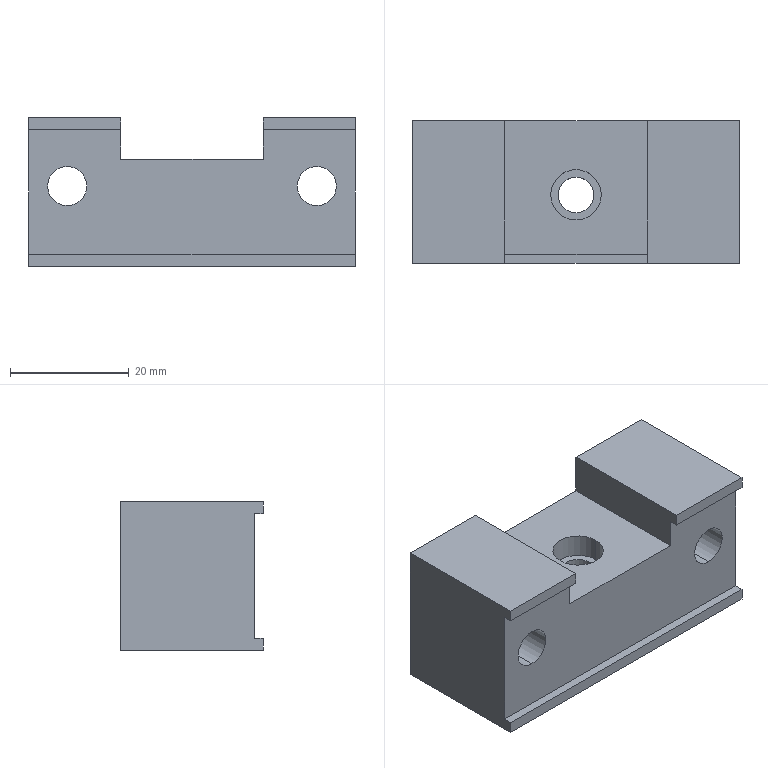Part | STEP file | 11-FG-B02711 | 1 solid | 39 faces | box 55 x 24 x 25 mm | volume 23943 mm3 | plane 21 | cylinder 18 | commonest cylinder face diameters 8.5 x6 6.6 x4 11 x4 4.2 x2 6 x2
STEP:
#1=CARTESIAN_POINT('',(18.75,15.,3.5));
#2=VERTEX_POINT('',#1);
#3=CARTESIAN_POINT('',(10.25,15.,3.5));
#4=VERTEX_POINT('',#3);
#5=CARTESIAN_POINT('',(14.5,15.,3.5));
#6=DIRECTION('',(0.,0.,-1.));
#7=DIRECTION('',(-1.,0.,0.));
#8=AXIS2_PLACEMENT_3D('',#5,#6,#7);
#9=CIRCLE('',#8,4.25);
#10=EDGE_CURVE('',#2,#4,#9,.T.);
#11=ORIENTED_EDGE('',*,*,#10,.F.);
#12=CARTESIAN_POINT('',(18.75,15.,0.));
#13=VERTEX_POINT('',#12);
#14=CARTESIAN_POINT('',(18.75,15.,3.5));
#15=DIRECTION('',(0.,0.,-1.));
#16=VECTOR('',#15,1000.);
#17=LINE('',#14,#16);
#18=EDGE_CURVE('',#2,#13,#17,.T.);
#19=ORIENTED_EDGE('',*,*,#18,.T.);
#20=CARTESIAN_POINT('',(10.25,15.,0.));
#21=VERTEX_POINT('',#20);
#22=CARTESIAN_POINT('',(14.5,15.,0.));
#23=DIRECTION('',(0.,0.,-1.));
#24=DIRECTION('',(-1.,0.,0.));
#25=AXIS2_PLACEMENT_3D('',#22,#23,#24);
#26=CIRCLE('',#25,4.25);
#27=EDGE_CURVE('',#13,#21,#26,.T.);
#28=ORIENTED_EDGE('',*,*,#27,.T.);
#29=CARTESIAN_POINT('',(10.25,15.,3.5));
#30=DIRECTION('',(0.,0.,-1.));
#31=VECTOR('',#30,1000.);
#32=LINE('',#29,#31);
#33=EDGE_CURVE('',#4,#21,#32,.T.);
#34=ORIENTED_EDGE('',*,*,#33,.F.);
#35=EDGE_LOOP('',(#11,#19,#28,#34));
#36=FACE_OUTER_BOUND('',#35,.T.);
#37=CARTESIAN_POINT('',(14.5,15.,3.5));
#38=DIRECTION('',(0.,0.,-1.));
#39=DIRECTION('',(-1.,0.,0.));
#40=AXIS2_PLACEMENT_3D('',#37,#38,#39);
#41=CYLINDRICAL_SURFACE('',#40,4.25);
#42=ADVANCED_FACE('',(#36),#41,.F.);
#43=CARTESIAN_POINT('',(44.75,15.,3.5));
#44=VERTEX_POINT('',#43);
#45=CARTESIAN_POINT('',(36.25,15.,3.5));
#46=VERTEX_POINT('',#45);
#47=CARTESIAN_POINT('',(40.5,15.,3.5));
#48=DIRECTION('',(0.,0.,-1.));
#49=DIRECTION('',(-1.,0.,0.));
#50=AXIS2_PLACEMENT_3D('',#47,#48,#49);
#51=CIRCLE('',#50,4.25);
#52=EDGE_CURVE('',#44,#46,#51,.T.);
#53=ORIENTED_EDGE('',*,*,#52,.F.);
#54=CARTESIAN_POINT('',(44.75,15.,0.));
#55=VERTEX_POINT('',#54);
#56=CARTESIAN_POINT('',(44.75,15.,3.5));
#57=DIRECTION('',(0.,0.,-1.));
#58=VECTOR('',#57,1000.);
#59=LINE('',#56,#58);
#60=EDGE_CURVE('',#44,#55,#59,.T.);
#61=ORIENTED_EDGE('',*,*,#60,.T.);
#62=CARTESIAN_POINT('',(36.25,15.,0.));
#63=VERTEX_POINT('',#62);
#64=CARTESIAN_POINT('',(40.5,15.,0.));
#65=DIRECTION('',(0.,0.,-1.));
#66=DIRECTION('',(-1.,0.,0.));
#67=AXIS2_PLACEMENT_3D('',#64,#65,#66);
#68=CIRCLE('',#67,4.25);
#69=EDGE_CURVE('',#55,#63,#68,.T.);
#70=ORIENTED_EDGE('',*,*,#69,.T.);
#71=CARTESIAN_POINT('',(36.25,15.,3.5));
#72=DIRECTION('',(0.,0.,-1.));
#73=VECTOR('',#72,1000.);
#74=LINE('',#71,#73);
#75=EDGE_CURVE('',#46,#63,#74,.T.);
#76=ORIENTED_EDGE('',*,*,#75,.F.);
#77=EDGE_LOOP('',(#53,#61,#70,#76));
#78=FACE_OUTER_BOUND('',#77,.T.);
#79=CARTESIAN_POINT('',(40.5,15.,3.5));
#80=DIRECTION('',(0.,0.,-1.));
#81=DIRECTION('',(-1.,0.,0.));
#82=AXIS2_PLACEMENT_3D('',#79,#80,#81);
#83=CYLINDRICAL_SURFACE('',#82,4.25);
#84=ADVANCED_FACE('',(#78),#83,.F.);
#85=CARTESIAN_POINT('',(6.5,17.6,8.));
#86=VERTEX_POINT('',#85);
#87=CARTESIAN_POINT('',(6.5,17.6,19.));
#88=VERTEX_POINT('',#87);
#89=CARTESIAN_POINT('',(6.5,17.6,13.5));
#90=DIRECTION('',(0.,1.,0.));
#91=DIRECTION('',(0.,0.,1.));
#92=AXIS2_PLACEMENT_3D('',#89,#90,#91);
#93=CIRCLE('',#92,5.5);
#94=EDGE_CURVE('',#86,#88,#93,.T.);
#95=ORIENTED_EDGE('',*,*,#94,.F.);
#96=CARTESIAN_POINT('',(6.5,24.,8.));
#97=VERTEX_POINT('',#96);
#98=CARTESIAN_POINT('',(6.5,24.,8.));
#99=DIRECTION('',(0.,1.,0.));
#100=VECTOR('',#99,1000.);
#101=LINE('',#98,#100);
#102=EDGE_CURVE('',#86,#97,#101,.T.);
#103=ORIENTED_EDGE('',*,*,#102,.T.);
#104=CARTESIAN_POINT('',(6.5,24.,19.));
#105=VERTEX_POINT('',#104);
#106=CARTESIAN_POINT('',(6.5,24.,13.5));
#107=DIRECTION('',(0.,1.,0.));
#108=DIRECTION('',(0.,0.,1.));
#109=AXIS2_PLACEMENT_3D('',#106,#107,#108);
#110=CIRCLE('',#109,5.5);
#111=EDGE_CURVE('',#97,#105,#110,.T.);
#112=ORIENTED_EDGE('',*,*,#111,.T.);
#113=CARTESIAN_POINT('',(6.5,24.,19.));
#114=DIRECTION('',(0.,1.,0.));
#115=VECTOR('',#114,1000.);
#116=LINE('',#113,#115);
#117=EDGE_CURVE('',#88,#105,#116,.T.);
#118=ORIENTED_EDGE('',*,*,#117,.F.);
#119=EDGE_LOOP('',(#95,#103,#112,#118));
#120=FACE_OUTER_BOUND('',#119,.T.);
#121=CARTESIAN_POINT('',(6.5,24.,13.5));
#122=DIRECTION('',(0.,1.,0.));
#123=DIRECTION('',(0.,0.,1.));
#124=AXIS2_PLACEMENT_3D('',#121,#122,#123);
#125=CYLINDRICAL_SURFACE('',#124,5.5);
#126=ADVANCED_FACE('',(#120),#125,.F.);
#127=CARTESIAN_POINT('',(6.5,1.5,10.2));
#128=VERTEX_POINT('',#127);
#129=CARTESIAN_POINT('',(6.5,1.5,16.8));
#130=VERTEX_POINT('',#129);
#131=CARTESIAN_POINT('',(6.5,1.5,13.5));
#132=DIRECTION('',(0.,1.,0.));
#133=DIRECTION('',(-1.,0.,0.));
#134=AXIS2_PLACEMENT_3D('',#131,#132,#133);
#135=CIRCLE('',#134,3.3);
#136=EDGE_CURVE('',#128,#130,#135,.T.);
#137=ORIENTED_EDGE('',*,*,#136,.F.);
#138=CARTESIAN_POINT('',(6.5,17.6,10.2));
#139=VERTEX_POINT('',#138);
#140=CARTESIAN_POINT('',(6.5,24.,10.2));
#141=DIRECTION('',(0.,1.,0.));
#142=VECTOR('',#141,1000.);
#143=LINE('',#140,#142);
#144=EDGE_CURVE('',#128,#139,#143,.T.);
#145=ORIENTED_EDGE('',*,*,#144,.T.);
#146=CARTESIAN_POINT('',(6.5,17.6,16.8));
#147=VERTEX_POINT('',#146);
#148=CARTESIAN_POINT('',(6.5,17.6,13.5));
#149=DIRECTION('',(0.,1.,0.));
#150=DIRECTION('',(0.,0.,1.));
#151=AXIS2_PLACEMENT_3D('',#148,#149,#150);
#152=CIRCLE('',#151,3.3);
#153=EDGE_CURVE('',#139,#147,#152,.T.);
#154=ORIENTED_EDGE('',*,*,#153,.T.);
#155=CARTESIAN_POINT('',(6.5,24.,16.8));
#156=DIRECTION('',(0.,1.,0.));
#157=VECTOR('',#156,1000.);
#158=LINE('',#155,#157);
#159=EDGE_CURVE('',#130,#147,#158,.T.);
#160=ORIENTED_EDGE('',*,*,#159,.F.);
#161=EDGE_LOOP('',(#137,#145,#154,#160));
#162=FACE_OUTER_BOUND('',#161,.T.);
#163=CARTESIAN_POINT('',(6.5,24.,13.5));
#164=DIRECTION('',(0.,1.,0.));
#165=DIRECTION('',(0.,0.,1.));
#166=AXIS2_PLACEMENT_3D('',#163,#164,#165);
#167=CYLINDRICAL_SURFACE('',#166,3.3);
#168=ADVANCED_FACE('',(#162),#167,.F.);
#169=CARTESIAN_POINT('',(48.5,17.6,8.));
#170=VERTEX_POINT('',#169);
#171=CARTESIAN_POINT('',(48.5,17.6,19.));
#172=VERTEX_POINT('',#171);
#173=CARTESIAN_POINT('',(48.5,17.6,13.5));
#174=DIRECTION('',(0.,1.,0.));
#175=DIRECTION('',(0.,0.,1.));
#176=AXIS2_PLACEMENT_3D('',#173,#174,#175);
#177=CIRCLE('',#176,5.5);
#178=EDGE_CURVE('',#170,#172,#177,.T.);
#179=ORIENTED_EDGE('',*,*,#178,.F.);
#180=CARTESIAN_POINT('',(48.5,24.,8.));
#181=VERTEX_POINT('',#180);
#182=CARTESIAN_POINT('',(48.5,24.,8.));
#183=DIRECTION('',(0.,1.,0.));
#184=VECTOR('',#183,1000.);
#185=LINE('',#182,#184);
#186=EDGE_CURVE('',#170,#181,#185,.T.);
#187=ORIENTED_EDGE('',*,*,#186,.T.);
#188=CARTESIAN_POINT('',(48.5,24.,19.));
#189=VERTEX_POINT('',#188);
#190=CARTESIAN_POINT('',(48.5,24.,13.5));
#191=DIRECTION('',(0.,1.,0.));
#192=DIRECTION('',(0.,0.,1.));
#193=AXIS2_PLACEMENT_3D('',#190,#191,#192);
#194=CIRCLE('',#193,5.5);
#195=EDGE_CURVE('',#181,#189,#194,.T.);
#196=ORIENTED_EDGE('',*,*,#195,.T.);
#197=CARTESIAN_POINT('',(48.5,24.,19.));
#198=DIRECTION('',(0.,1.,0.));
#199=VECTOR('',#198,1000.);
#200=LINE('',#197,#199);
#201=EDGE_CURVE('',#172,#189,#200,.T.);
#202=ORIENTED_EDGE('',*,*,#201,.F.);
#203=EDGE_LOOP('',(#179,#187,#196,#202));
#204=FACE_OUTER_BOUND('',#203,.T.);
#205=CARTESIAN_POINT('',(48.5,24.,13.5));
#206=DIRECTION('',(0.,1.,0.));
#207=DIRECTION('',(0.,0.,1.));
#208=AXIS2_PLACEMENT_3D('',#205,#206,#207);
#209=CYLINDRICAL_SURFACE('',#208,5.5);
#210=ADVANCED_FACE('',(#204),#209,.F.);
#211=CARTESIAN_POINT('',(48.5,1.5,10.2));
#212=VERTEX_POINT('',#211);
#213=CARTESIAN_POINT('',(48.5,1.5,16.8));
#214=VERTEX_POINT('',#213);
#215=CARTESIAN_POINT('',(48.5,1.5,13.5));
#216=DIRECTION('',(0.,1.,0.));
#217=DIRECTION('',(-1.,0.,0.));
#218=AXIS2_PLACEMENT_3D('',#215,#216,#217);
#219=CIRCLE('',#218,3.3);
#220=EDGE_CURVE('',#212,#214,#219,.T.);
#221=ORIENTED_EDGE('',*,*,#220,.F.);
#222=CARTESIAN_POINT('',(48.5,17.6,10.2));
#223=VERTEX_POINT('',#222);
#224=CARTESIAN_POINT('',(48.5,24.,10.2));
#225=DIRECTION('',(0.,1.,0.));
#226=VECTOR('',#225,1000.);
#227=LINE('',#224,#226);
#228=EDGE_CURVE('',#212,#223,#227,.T.);
#229=ORIENTED_EDGE('',*,*,#228,.T.);
#230=CARTESIAN_POINT('',(48.5,17.6,16.8));
#231=VERTEX_POINT('',#230);
#232=CARTESIAN_POINT('',(48.5,17.6,13.5));
#233=DIRECTION('',(0.,1.,0.));
#234=DIRECTION('',(0.,0.,1.));
#235=AXIS2_PLACEMENT_3D('',#232,#233,#234);
#236=CIRCLE('',#235,3.3);
#237=EDGE_CURVE('',#223,#231,#236,.T.);
#238=ORIENTED_EDGE('',*,*,#237,.T.);
#239=CARTESIAN_POINT('',(48.5,24.,16.8));
#240=DIRECTION('',(0.,1.,0.));
#241=VECTOR('',#240,1000.);
#242=LINE('',#239,#241);
#243=EDGE_CURVE('',#214,#231,#242,.T.);
#244=ORIENTED_EDGE('',*,*,#243,.F.);
#245=EDGE_LOOP('',(#221,#229,#238,#244));
#246=FACE_OUTER_BOUND('',#245,.T.);
#247=CARTESIAN_POINT('',(48.5,24.,13.5));
#248=DIRECTION('',(0.,1.,0.));
#249=DIRECTION('',(0.,0.,1.));
#250=AXIS2_PLACEMENT_3D('',#247,#248,#249);
#251=CYLINDRICAL_SURFACE('',#250,3.3);
#252=ADVANCED_FACE('',(#246),#251,.F.);
#253=CARTESIAN_POINT('',(27.5,14.5,2.4));
#254=VERTEX_POINT('',#253);
#255=CARTESIAN_POINT('',(27.5,14.5,6.6));
#256=VERTEX_POINT('',#255);
#257=CARTESIAN_POINT('',(27.5,14.5,2.4));
#258=CARTESIAN_POINT('',(27.358,14.5,2.4));
#259=CARTESIAN_POINT('',(27.214,14.49,2.415));
#260=CARTESIAN_POINT('',(26.936,14.45,2.472));
#261=CARTESIAN_POINT('',(26.803,14.421,2.514));
#262=CARTESIAN_POINT('',(26.419,14.311,2.678));
#263=CARTESIAN_POINT('',(26.194,14.209,2.834));
#264=CARTESIAN_POINT('',(25.915,14.049,3.116));
#265=CARTESIAN_POINT('',(25.831,13.995,3.218));
#266=CARTESIAN_POINT('',(25.683,13.889,3.439));
#267=CARTESIAN_POINT('',(25.618,13.837,3.558));
#268=CARTESIAN_POINT('',(25.513,13.749,3.807));
#269=CARTESIAN_POINT('',(25.471,13.71,3.941));
#270=CARTESIAN_POINT('',(25.414,13.657,4.217));
#271=CARTESIAN_POINT('',(25.4,13.642,4.358));
#272=CARTESIAN_POINT('',(25.4,13.643,4.647));
#273=CARTESIAN_POINT('',(25.415,13.658,4.788));
#274=CARTESIAN_POINT('',(25.472,13.711,5.064));
#275=CARTESIAN_POINT('',(25.515,13.75,5.197));
#276=CARTESIAN_POINT('',(25.673,13.884,5.571));
#277=CARTESIAN_POINT('',(25.824,13.998,5.793));
#278=CARTESIAN_POINT('',(26.105,14.158,6.075));
#279=CARTESIAN_POINT('',(26.209,14.211,6.162));
#280=CARTESIAN_POINT('',(26.431,14.305,6.312));
#281=CARTESIAN_POINT('',(26.549,14.348,6.377));
#282=CARTESIAN_POINT('',(26.803,14.421,6.486));
#283=CARTESIAN_POINT('',(26.939,14.45,6.528));
#284=CARTESIAN_POINT('',(27.214,14.49,6.585));
#285=CARTESIAN_POINT('',(27.356,14.5,6.6));
#286=CARTESIAN_POINT('',(27.5,14.5,6.6));
#287=B_SPLINE_CURVE_WITH_KNOTS('',3,(#257,#258,#259,#260,#261,#262,#263,#264,#265,#266,#267,#268,#269,#270,#271,#272,#273,#274,#275,#276,#277,#278,#279,#280,#281,#282,#283,#284,#285,#286),.UNSPECIFIED.,.F.,.F.,(4,2,2,2,2,2,2,2,2,2,2,2,2,2,4),(0.006821,0.007247,0.007673,0.008524,0.00895,0.009376,0.009801,0.01023,0.01065,0.01108,0.01193,0.01236,0.01278,0.01321,0.01363),.UNSPECIFIED.);
#288=EDGE_CURVE('',#254,#256,#287,.T.);
#289=ORIENTED_EDGE('',*,*,#288,.F.);
#290=CARTESIAN_POINT('',(27.5,24.,2.4));
#291=VERTEX_POINT('',#290);
#292=CARTESIAN_POINT('',(27.5,24.,2.4));
#293=DIRECTION('',(0.,1.,0.));
#294=VECTOR('',#293,1000.);
#295=LINE('',#292,#294);
#296=EDGE_CURVE('',#254,#291,#295,.T.);
#297=ORIENTED_EDGE('',*,*,#296,.T.);
#298=CARTESIAN_POINT('',(27.5,24.,6.6));
#299=VERTEX_POINT('',#298);
#300=CARTESIAN_POINT('',(27.5,24.,4.5));
#301=DIRECTION('',(0.,1.,0.));
#302=DIRECTION('',(0.,0.,1.));
#303=AXIS2_PLACEMENT_3D('',#300,#301,#302);
#304=CIRCLE('',#303,2.1);
#305=EDGE_CURVE('',#291,#299,#304,.T.);
#306=ORIENTED_EDGE('',*,*,#305,.T.);
#307=CARTESIAN_POINT('',(27.5,24.,6.6));
#308=DIRECTION('',(0.,1.,0.));
#309=VECTOR('',#308,1000.);
#310=LINE('',#307,#309);
#311=EDGE_CURVE('',#256,#299,#310,.T.);
#312=ORIENTED_EDGE('',*,*,#311,.F.);
#313=EDGE_LOOP('',(#289,#297,#306,#312));
#314=FACE_OUTER_BOUND('',#313,.T.);
#315=CARTESIAN_POINT('',(27.5,24.,4.5));
#316=DIRECTION('',(0.,1.,0.));
#317=DIRECTION('',(0.,0.,1.));
#318=AXIS2_PLACEMENT_3D('',#315,#316,#317);
#319=CYLINDRICAL_SURFACE('',#318,2.1);
#320=ADVANCED_FACE('',(#314),#319,.F.);
#321=CARTESIAN_POINT('',(23.25,11.5,14.));
#322=VERTEX_POINT('',#321);
#323=CARTESIAN_POINT('',(31.75,11.5,14.));
#324=VERTEX_POINT('',#323);
#325=CARTESIAN_POINT('',(27.5,11.5,14.));
#326=DIRECTION('',(0.,0.,1.));
#327=DIRECTION('',(1.,0.,0.));
#328=AXIS2_PLACEMENT_3D('',#325,#326,#327);
#329=CIRCLE('',#328,4.25);
#330=EDGE_CURVE('',#322,#324,#329,.T.);
#331=ORIENTED_EDGE('',*,*,#330,.F.);
#332=CARTESIAN_POINT('',(23.25,11.5,18.));
#333=VERTEX_POINT('',#332);
#334=CARTESIAN_POINT('',(23.25,11.5,14.));
#335=DIRECTION('',(0.,0.,1.));
#336=VECTOR('',#335,1000.);
#337=LINE('',#334,#336);
#338=EDGE_CURVE('',#322,#333,#337,.T.);
#339=ORIENTED_EDGE('',*,*,#338,.T.);
#340=CARTESIAN_POINT('',(31.75,11.5,18.));
#341=VERTEX_POINT('',#340);
#342=CARTESIAN_POINT('',(27.5,11.5,18.));
#343=DIRECTION('',(0.,0.,1.));
#344=DIRECTION('',(1.,0.,0.));
#345=AXIS2_PLACEMENT_3D('',#342,#343,#344);
#346=CIRCLE('',#345,4.25);
#347=EDGE_CURVE('',#333,#341,#346,.T.);
#348=ORIENTED_EDGE('',*,*,#347,.T.);
#349=CARTESIAN_POINT('',(31.75,11.5,14.));
#350=DIRECTION('',(0.,0.,1.));
#351=VECTOR('',#350,1000.);
#352=LINE('',#349,#351);
#353=EDGE_CURVE('',#324,#341,#352,.T.);
#354=ORIENTED_EDGE('',*,*,#353,.F.);
#355=EDGE_LOOP('',(#331,#339,#348,#354));
#356=FACE_OUTER_BOUND('',#355,.T.);
#357=CARTESIAN_POINT('',(27.5,11.5,14.));
#358=DIRECTION('',(0.,0.,1.));
#359=DIRECTION('',(1.,0.,0.));
#360=AXIS2_PLACEMENT_3D('',#357,#358,#359);
#361=CYLINDRICAL_SURFACE('',#360,4.25);
#362=ADVANCED_FACE('',(#356),#361,.F.);
#363=CARTESIAN_POINT('',(30.5,11.5,0.));
#364=VERTEX_POINT('',#363);
#365=CARTESIAN_POINT('',(24.5,11.5,0.));
#366=VERTEX_POINT('',#365);
#367=CARTESIAN_POINT('',(27.5,11.5,0.));
#368=DIRECTION('',(0.,0.,-1.));
#369=DIRECTION('',(-1.,0.,0.));
#370=AXIS2_PLACEMENT_3D('',#367,#368,#369);
#371=CIRCLE('',#370,3.);
#372=EDGE_CURVE('',#364,#366,#371,.T.);
#373=ORIENTED_EDGE('',*,*,#372,.T.);
#374=CARTESIAN_POINT('',(24.5,11.5,14.));
#375=VERTEX_POINT('',#374);
#376=CARTESIAN_POINT('',(24.5,11.5,-89.));
#377=DIRECTION('',(0.,0.,1.));
#378=VECTOR('',#377,1000.);
#379=LINE('',#376,#378);
#380=EDGE_CURVE('',#366,#375,#379,.T.);
#381=ORIENTED_EDGE('',*,*,#380,.T.);
#382=CARTESIAN_POINT('',(30.5,11.5,14.));
#383=VERTEX_POINT('',#382);
#384=CARTESIAN_POINT('',(27.5,11.5,14.));
#385=DIRECTION('',(0.,0.,-1.));
#386=DIRECTION('',(1.,0.,0.));
#387=AXIS2_PLACEMENT_3D('',#384,#385,#386);
#388=CIRCLE('',#387,3.);
#389=EDGE_CURVE('',#383,#375,#388,.T.);
#390=ORIENTED_EDGE('',*,*,#389,.F.);
#391=CARTESIAN_POINT('',(30.5,11.5,-89.));
#392=DIRECTION('',(0.,0.,1.));
#393=VECTOR('',#392,1000.);
#394=LINE('',#391,#393);
#395=EDGE_CURVE('',#364,#383,#394,.T.);
#396=ORIENTED_EDGE('',*,*,#395,.F.);
#397=EDGE_LOOP('',(#373,#381,#390,#396));
#398=FACE_OUTER_BOUND('',#397,.T.);
#399=CARTESIAN_POINT('',(27.5,11.5,-89.));
#400=DIRECTION('',(0.,0.,1.));
#401=DIRECTION('',(1.,0.,0.));
#402=AXIS2_PLACEMENT_3D('',#399,#400,#401);
#403=CYLINDRICAL_SURFACE('',#402,3.);
#404=ADVANCED_FACE('',(#398),#403,.F.);
#405=ORIENTED_EDGE('',*,*,#380,.F.);
#406=CARTESIAN_POINT('',(27.5,11.5,0.));
#407=DIRECTION('',(0.,0.,-1.));
#408=DIRECTION('',(-1.,0.,0.));
#409=AXIS2_PLACEMENT_3D('',#406,#407,#408);
#410=CIRCLE('',#409,3.);
#411=EDGE_CURVE('',#366,#364,#410,.T.);
#412=ORIENTED_EDGE('',*,*,#411,.T.);
#413=ORIENTED_EDGE('',*,*,#395,.T.);
#414=CARTESIAN_POINT('',(27.5,11.5,14.));
#415=DIRECTION('',(0.,0.,-1.));
#416=DIRECTION('',(1.,0.,0.));
#417=AXIS2_PLACEMENT_3D('',#414,#415,#416);
#418=CIRCLE('',#417,3.);
#419=EDGE_CURVE('',#375,#383,#418,.T.);
#420=ORIENTED_EDGE('',*,*,#419,.F.);
#421=EDGE_LOOP('',(#405,#412,#413,#420));
#422=FACE_OUTER_BOUND('',#421,.T.);
#423=CARTESIAN_POINT('',(27.5,14.5,6.6));
#424=CARTESIAN_POINT('',(27.644,14.5,6.6));
#425=CARTESIAN_POINT('',(27.786,14.49,6.585));
#426=CARTESIAN_POINT('',(28.062,14.45,6.528));
#427=CARTESIAN_POINT('',(28.198,14.421,6.485));
#428=CARTESIAN_POINT('',(28.578,14.312,6.323));
#429=CARTESIAN_POINT('',(28.804,14.21,6.167));
#430=CARTESIAN_POINT('',(29.084,14.05,5.885));
#431=CARTESIAN_POINT('',(29.169,13.995,5.782));
#432=CARTESIAN_POINT('',(29.316,13.889,5.562));
#433=CARTESIAN_POINT('',(29.38,13.839,5.446));
#434=CARTESIAN_POINT('',(29.486,13.75,5.196));
#435=CARTESIAN_POINT('',(29.528,13.711,5.062));
#436=CARTESIAN_POINT('',(29.585,13.657,4.788));
#437=CARTESIAN_POINT('',(29.6,13.642,4.643));
#438=CARTESIAN_POINT('',(29.6,13.642,4.358));
#439=CARTESIAN_POINT('',(29.586,13.657,4.216));
#440=CARTESIAN_POINT('',(29.528,13.711,3.938));
#441=CARTESIAN_POINT('',(29.487,13.749,3.807));
#442=CARTESIAN_POINT('',(29.327,13.884,3.429));
#443=CARTESIAN_POINT('',(29.179,13.996,3.21));
#444=CARTESIAN_POINT('',(28.897,14.157,2.926));
#445=CARTESIAN_POINT('',(28.795,14.209,2.841));
#446=CARTESIAN_POINT('',(28.573,14.304,2.69));
#447=CARTESIAN_POINT('',(28.453,14.348,2.624));
#448=CARTESIAN_POINT('',(28.198,14.421,2.514));
#449=CARTESIAN_POINT('',(28.064,14.45,2.472));
#450=CARTESIAN_POINT('',(27.787,14.49,2.415));
#451=CARTESIAN_POINT('',(27.642,14.5,2.4));
#452=CARTESIAN_POINT('',(27.5,14.5,2.4));
#453=B_SPLINE_CURVE_WITH_KNOTS('',3,(#423,#424,#425,#426,#427,#428,#429,#430,#431,#432,#433,#434,#435,#436,#437,#438,#439,#440,#441,#442,#443,#444,#445,#446,#447,#448,#449,#450,#451,#452),.UNSPECIFIED.,.F.,.F.,(4,2,2,2,2,2,2,2,2,2,2,2,2,2,4),(0.,0.0004263,0.0008526,0.001705,0.002132,0.002558,0.002984,0.003411,0.003837,0.004263,0.005116,0.005542,0.005969,0.006395,0.006821),.UNSPECIFIED.);
#454=EDGE_CURVE('',#256,#254,#453,.T.);
#455=ORIENTED_EDGE('',*,*,#454,.T.);
#456=ORIENTED_EDGE('',*,*,#288,.T.);
#457=EDGE_LOOP('',(#455,#456));
#458=FACE_BOUND('',#457,.T.);
#459=CARTESIAN_POINT('',(27.5,11.5,-89.));
#460=DIRECTION('',(0.,0.,1.));
#461=DIRECTION('',(1.,0.,0.));
#462=AXIS2_PLACEMENT_3D('',#459,#460,#461);
#463=CYLINDRICAL_SURFACE('',#462,3.);
#464=ADVANCED_FACE('',(#422,#458),#463,.F.);
#465=CARTESIAN_POINT('',(39.5,0.,25.));
#466=VERTEX_POINT('',#465);
#467=CARTESIAN_POINT('',(55.,0.,25.));
#468=VERTEX_POINT('',#467);
#469=CARTESIAN_POINT('',(0.,0.,25.));
#470=DIRECTION('',(1.,0.,0.));
#471=VECTOR('',#470,1000.);
#472=LINE('',#469,#471);
#473=EDGE_CURVE('',#466,#468,#472,.T.);
#474=ORIENTED_EDGE('',*,*,#473,.F.);
#475=CARTESIAN_POINT('',(39.5,0.,23.));
#476=VERTEX_POINT('',#475);
#477=CARTESIAN_POINT('',(39.5,0.,25.));
#478=DIRECTION('',(0.,0.,-1.));
#479=VECTOR('',#478,1000.);
#480=LINE('',#477,#479);
#481=EDGE_CURVE('',#466,#476,#480,.T.);
#482=ORIENTED_EDGE('',*,*,#481,.T.);
#483=CARTESIAN_POINT('',(55.,0.,23.));
#484=VERTEX_POINT('',#483);
#485=CARTESIAN_POINT('',(107.,0.,23.));
#486=DIRECTION('',(-1.,0.,0.));
#487=VECTOR('',#486,1000.);
#488=LINE('',#485,#487);
#489=EDGE_CURVE('',#484,#476,#488,.T.);
#490=ORIENTED_EDGE('',*,*,#489,.F.);
#491=CARTESIAN_POINT('',(55.,0.,25.));
#492=DIRECTION('',(0.,0.,-1.));
#493=VECTOR('',#492,1000.);
#494=LINE('',#491,#493);
#495=EDGE_CURVE('',#468,#484,#494,.T.);
#496=ORIENTED_EDGE('',*,*,#495,.F.);
#497=EDGE_LOOP('',(#474,#482,#490,#496));
#498=FACE_OUTER_BOUND('',#497,.T.);
#499=CARTESIAN_POINT('',(0.,0.,25.));
#500=DIRECTION('',(0.,1.,0.));
#501=DIRECTION('',(0.,0.,1.));
#502=AXIS2_PLACEMENT_3D('',#499,#500,#501);
#503=PLANE('',#502);
#504=ADVANCED_FACE('',(#498),#503,.F.);
#505=CARTESIAN_POINT('',(55.,24.,25.));
#506=VERTEX_POINT('',#505);
#507=CARTESIAN_POINT('',(39.5,24.,25.));
#508=VERTEX_POINT('',#507);
#509=CARTESIAN_POINT('',(0.,24.,25.));
#510=DIRECTION('',(-1.,0.,0.));
#511=VECTOR('',#510,1000.);
#512=LINE('',#509,#511);
#513=EDGE_CURVE('',#506,#508,#512,.T.);
#514=ORIENTED_EDGE('',*,*,#513,.T.);
#515=CARTESIAN_POINT('',(39.5,-83.,25.));
#516=DIRECTION('',(0.,1.,0.));
#517=VECTOR('',#516,1000.);
#518=LINE('',#515,#517);
#519=EDGE_CURVE('',#466,#508,#518,.T.);
#520=ORIENTED_EDGE('',*,*,#519,.F.);
#521=ORIENTED_EDGE('',*,*,#473,.T.);
#522=CARTESIAN_POINT('',(55.,0.,25.));
#523=DIRECTION('',(0.,1.,0.));
#524=VECTOR('',#523,1000.);
#525=LINE('',#522,#524);
#526=EDGE_CURVE('',#468,#506,#525,.T.);
#527=ORIENTED_EDGE('',*,*,#526,.T.);
#528=EDGE_LOOP('',(#514,#520,#521,#527));
#529=FACE_OUTER_BOUND('',#528,.T.);
#530=CARTESIAN_POINT('',(0.,24.,25.));
#531=DIRECTION('',(0.,0.,-1.));
#532=DIRECTION('',(-1.,0.,0.));
#533=AXIS2_PLACEMENT_3D('',#530,#531,#532);
#534=PLANE('',#533);
#535=ADVANCED_FACE('',(#529),#534,.F.);
#536=ORIENTED_EDGE('',*,*,#489,.T.);
#537=CARTESIAN_POINT('',(39.5,1.5,23.));
#538=VERTEX_POINT('',#537);
#539=CARTESIAN_POINT('',(39.5,0.,23.));
#540=DIRECTION('',(0.,1.,0.));
#541=VECTOR('',#540,1000.);
#542=LINE('',#539,#541);
#543=EDGE_CURVE('',#476,#538,#542,.T.);
#544=ORIENTED_EDGE('',*,*,#543,.T.);
#545=CARTESIAN_POINT('',(55.,1.5,23.));
#546=VERTEX_POINT('',#545);
#547=CARTESIAN_POINT('',(107.,1.5,23.));
#548=DIRECTION('',(-1.,0.,0.));
#549=VECTOR('',#548,1000.);
#550=LINE('',#547,#549);
#551=EDGE_CURVE('',#546,#538,#550,.T.);
#552=ORIENTED_EDGE('',*,*,#551,.F.);
#553=CARTESIAN_POINT('',(55.,0.,23.));
#554=DIRECTION('',(0.,1.,0.));
#555=VECTOR('',#554,1000.);
#556=LINE('',#553,#555);
#557=EDGE_CURVE('',#484,#546,#556,.T.);
#558=ORIENTED_EDGE('',*,*,#557,.F.);
#559=EDGE_LOOP('',(#536,#544,#552,#558));
#560=FACE_OUTER_BOUND('',#559,.T.);
#561=CARTESIAN_POINT('',(107.,0.,23.));
#562=DIRECTION('',(0.,0.,1.));
#563=DIRECTION('',(1.,0.,0.));
#564=AXIS2_PLACEMENT_3D('',#561,#562,#563);
#565=PLANE('',#564);
#566=ADVANCED_FACE('',(#560),#565,.F.);
#567=CARTESIAN_POINT('',(15.5,0.,23.));
#568=VERTEX_POINT('',#567);
#569=CARTESIAN_POINT('',(0.,0.,23.));
#570=VERTEX_POINT('',#569);
#571=CARTESIAN_POINT('',(107.,0.,23.));
#572=DIRECTION('',(-1.,0.,0.));
#573=VECTOR('',#572,1000.);
#574=LINE('',#571,#573);
#575=EDGE_CURVE('',#568,#570,#574,.T.);
#576=ORIENTED_EDGE('',*,*,#575,.F.);
#577=CARTESIAN_POINT('',(15.5,0.,25.));
#578=VERTEX_POINT('',#577);
#579=CARTESIAN_POINT('',(15.5,0.,25.));
#580=DIRECTION('',(0.,0.,1.));
#581=VECTOR('',#580,1000.);
#582=LINE('',#579,#581);
#583=EDGE_CURVE('',#568,#578,#582,.T.);
#584=ORIENTED_EDGE('',*,*,#583,.T.);
#585=CARTESIAN_POINT('',(0.,0.,25.));
#586=VERTEX_POINT('',#585);
#587=CARTESIAN_POINT('',(0.,0.,25.));
#588=DIRECTION('',(1.,0.,0.));
#589=VECTOR('',#588,1000.);
#590=LINE('',#587,#589);
#591=EDGE_CURVE('',#586,#578,#590,.T.);
#592=ORIENTED_EDGE('',*,*,#591,.F.);
#593=CARTESIAN_POINT('',(0.,0.,25.));
#594=DIRECTION('',(0.,0.,-1.));
#595=VECTOR('',#594,1000.);
#596=LINE('',#593,#595);
#597=EDGE_CURVE('',#586,#570,#596,.T.);
#598=ORIENTED_EDGE('',*,*,#597,.T.);
#599=EDGE_LOOP('',(#576,#584,#592,#598));
#600=FACE_OUTER_BOUND('',#599,.T.);
#601=CARTESIAN_POINT('',(0.,0.,25.));
#602=DIRECTION('',(0.,1.,0.));
#603=DIRECTION('',(0.,0.,1.));
#604=AXIS2_PLACEMENT_3D('',#601,#602,#603);
#605=PLANE('',#604);
#606=ADVANCED_FACE('',(#600),#605,.F.);
#607=CARTESIAN_POINT('',(0.,1.5,23.));
#608=VERTEX_POINT('',#607);
#609=CARTESIAN_POINT('',(0.,1.5,2.));
#610=VERTEX_POINT('',#609);
#611=CARTESIAN_POINT('',(0.,1.5,23.));
#612=DIRECTION('',(0.,0.,-1.));
#613=VECTOR('',#612,1000.);
#614=LINE('',#611,#613);
#615=EDGE_CURVE('',#608,#610,#614,.T.);
#616=ORIENTED_EDGE('',*,*,#615,.F.);
#617=CARTESIAN_POINT('',(0.,0.,23.));
#618=DIRECTION('',(0.,1.,0.));
#619=VECTOR('',#618,1000.);
#620=LINE('',#617,#619);
#621=EDGE_CURVE('',#570,#608,#620,.T.);
#622=ORIENTED_EDGE('',*,*,#621,.F.);
#623=ORIENTED_EDGE('',*,*,#597,.F.);
#624=CARTESIAN_POINT('',(0.,24.,25.));
#625=VERTEX_POINT('',#624);
#626=CARTESIAN_POINT('',(0.,0.,25.));
#627=DIRECTION('',(0.,-1.,0.));
#628=VECTOR('',#627,1000.);
#629=LINE('',#626,#628);
#630=EDGE_CURVE('',#625,#586,#629,.T.);
#631=ORIENTED_EDGE('',*,*,#630,.F.);
#632=CARTESIAN_POINT('',(0.,24.,0.));
#633=VERTEX_POINT('',#632);
#634=CARTESIAN_POINT('',(0.,24.,25.));
#635=DIRECTION('',(0.,0.,-1.));
#636=VECTOR('',#635,1000.);
#637=LINE('',#634,#636);
#638=EDGE_CURVE('',#625,#633,#637,.T.);
#639=ORIENTED_EDGE('',*,*,#638,.T.);
#640=CARTESIAN_POINT('',(0.,0.,0.));
#641=VERTEX_POINT('',#640);
#642=CARTESIAN_POINT('',(0.,0.,0.));
#643=DIRECTION('',(0.,-1.,0.));
#644=VECTOR('',#643,1000.);
#645=LINE('',#642,#644);
#646=EDGE_CURVE('',#633,#641,#645,.T.);
#647=ORIENTED_EDGE('',*,*,#646,.T.);
#648=CARTESIAN_POINT('',(0.,0.,2.));
#649=VERTEX_POINT('',#648);
#650=CARTESIAN_POINT('',(0.,0.,25.));
#651=DIRECTION('',(0.,0.,-1.));
#652=VECTOR('',#651,1000.);
#653=LINE('',#650,#652);
#654=EDGE_CURVE('',#649,#641,#653,.T.);
#655=ORIENTED_EDGE('',*,*,#654,.F.);
#656=CARTESIAN_POINT('',(0.,0.,2.));
#657=DIRECTION('',(0.,-1.,0.));
#658=VECTOR('',#657,1000.);
#659=LINE('',#656,#658);
#660=EDGE_CURVE('',#610,#649,#659,.T.);
#661=ORIENTED_EDGE('',*,*,#660,.F.);
#662=EDGE_LOOP('',(#616,#622,#623,#631,#639,#647,#655,#661));
#663=FACE_OUTER_BOUND('',#662,.T.);
#664=CARTESIAN_POINT('',(0.,0.,25.));
#665=DIRECTION('',(1.,0.,0.));
#666=DIRECTION('',(0.,1.,0.));
#667=AXIS2_PLACEMENT_3D('',#664,#665,#666);
#668=PLANE('',#667);
#669=ADVANCED_FACE('',(#663),#668,.F.);
#670=CARTESIAN_POINT('',(55.,0.,2.));
#671=VERTEX_POINT('',#670);
#672=CARTESIAN_POINT('',(55.,0.,0.));
#673=VERTEX_POINT('',#672);
#674=CARTESIAN_POINT('',(55.,0.,25.));
#675=DIRECTION('',(0.,0.,-1.));
#676=VECTOR('',#675,1000.);
#677=LINE('',#674,#676);
#678=EDGE_CURVE('',#671,#673,#677,.T.);
#679=ORIENTED_EDGE('',*,*,#678,.F.);
#680=CARTESIAN_POINT('',(107.,0.,2.));
#681=DIRECTION('',(-1.,0.,0.));
#682=VECTOR('',#681,1000.);
#683=LINE('',#680,#682);
#684=EDGE_CURVE('',#671,#649,#683,.T.);
#685=ORIENTED_EDGE('',*,*,#684,.T.);
#686=ORIENTED_EDGE('',*,*,#654,.T.);
#687=CARTESIAN_POINT('',(0.,0.,0.));
#688=DIRECTION('',(1.,0.,0.));
#689=VECTOR('',#688,1000.);
#690=LINE('',#687,#689);
#691=EDGE_CURVE('',#641,#673,#690,.T.);
#692=ORIENTED_EDGE('',*,*,#691,.T.);
#693=EDGE_LOOP('',(#679,#685,#686,#692));
#694=FACE_OUTER_BOUND('',#693,.T.);
#695=CARTESIAN_POINT('',(0.,0.,25.));
#696=DIRECTION('',(0.,1.,0.));
#697=DIRECTION('',(0.,0.,1.));
#698=AXIS2_PLACEMENT_3D('',#695,#696,#697);
#699=PLANE('',#698);
#700=ADVANCED_FACE('',(#694),#699,.F.);
#701=ORIENTED_EDGE('',*,*,#495,.T.);
#702=ORIENTED_EDGE('',*,*,#557,.T.);
#703=CARTESIAN_POINT('',(55.,1.5,2.));
#704=VERTEX_POINT('',#703);
#705=CARTESIAN_POINT('',(55.,1.5,25.));
#706=DIRECTION('',(0.,0.,-1.));
#707=VECTOR('',#706,1000.);
#708=LINE('',#705,#707);
#709=EDGE_CURVE('',#546,#704,#708,.T.);
#710=ORIENTED_EDGE('',*,*,#709,.T.);
#711=CARTESIAN_POINT('',(55.,0.,2.));
#712=DIRECTION('',(0.,-1.,0.));
#713=VECTOR('',#712,1000.);
#714=LINE('',#711,#713);
#715=EDGE_CURVE('',#704,#671,#714,.T.);
#716=ORIENTED_EDGE('',*,*,#715,.T.);
#717=ORIENTED_EDGE('',*,*,#678,.T.);
#718=CARTESIAN_POINT('',(55.,24.,0.));
#719=VERTEX_POINT('',#718);
#720=CARTESIAN_POINT('',(55.,0.,0.));
#721=DIRECTION('',(0.,1.,0.));
#722=VECTOR('',#721,1000.);
#723=LINE('',#720,#722);
#724=EDGE_CURVE('',#673,#719,#723,.T.);
#725=ORIENTED_EDGE('',*,*,#724,.T.);
#726=CARTESIAN_POINT('',(55.,24.,25.));
#727=DIRECTION('',(0.,0.,-1.));
#728=VECTOR('',#727,1000.);
#729=LINE('',#726,#728);
#730=EDGE_CURVE('',#506,#719,#729,.T.);
#731=ORIENTED_EDGE('',*,*,#730,.F.);
#732=ORIENTED_EDGE('',*,*,#526,.F.);
#733=EDGE_LOOP('',(#701,#702,#710,#716,#717,#725,#731,#732));
#734=FACE_OUTER_BOUND('',#733,.T.);
#735=CARTESIAN_POINT('',(55.,0.,25.));
#736=DIRECTION('',(-1.,0.,0.));
#737=DIRECTION('',(0.,-1.,0.));
#738=AXIS2_PLACEMENT_3D('',#735,#736,#737);
#739=PLANE('',#738);
#740=ADVANCED_FACE('',(#734),#739,.F.);
#741=CARTESIAN_POINT('',(6.5,24.,13.5));
#742=DIRECTION('',(0.,1.,0.));
#743=DIRECTION('',(0.,0.,1.));
#744=AXIS2_PLACEMENT_3D('',#741,#742,#743);
#745=CIRCLE('',#744,5.5);
#746=EDGE_CURVE('',#105,#97,#745,.T.);
#747=ORIENTED_EDGE('',*,*,#746,.F.);
#748=ORIENTED_EDGE('',*,*,#111,.F.);
#749=EDGE_LOOP('',(#747,#748));
#750=FACE_BOUND('',#749,.T.);
#751=CARTESIAN_POINT('',(48.5,24.,13.5));
#752=DIRECTION('',(0.,1.,0.));
#753=DIRECTION('',(0.,0.,1.));
#754=AXIS2_PLACEMENT_3D('',#751,#752,#753);
#755=CIRCLE('',#754,5.5);
#756=EDGE_CURVE('',#189,#181,#755,.T.);
#757=ORIENTED_EDGE('',*,*,#756,.F.);
#758=ORIENTED_EDGE('',*,*,#195,.F.);
#759=EDGE_LOOP('',(#757,#758));
#760=FACE_BOUND('',#759,.T.);
#761=CARTESIAN_POINT('',(27.5,24.,4.5));
#762=DIRECTION('',(0.,1.,0.));
#763=DIRECTION('',(0.,0.,1.));
#764=AXIS2_PLACEMENT_3D('',#761,#762,#763);
#765=CIRCLE('',#764,2.1);
#766=EDGE_CURVE('',#299,#291,#765,.T.);
#767=ORIENTED_EDGE('',*,*,#766,.F.);
#768=ORIENTED_EDGE('',*,*,#305,.F.);
#769=EDGE_LOOP('',(#767,#768));
#770=FACE_BOUND('',#769,.T.);
#771=CARTESIAN_POINT('',(39.5,24.,18.));
#772=VERTEX_POINT('',#771);
#773=CARTESIAN_POINT('',(15.5,24.,18.));
#774=VERTEX_POINT('',#773);
#775=CARTESIAN_POINT('',(39.5,24.,18.));
#776=DIRECTION('',(-1.,0.,0.));
#777=VECTOR('',#776,1000.);
#778=LINE('',#775,#777);
#779=EDGE_CURVE('',#772,#774,#778,.T.);
#780=ORIENTED_EDGE('',*,*,#779,.F.);
#781=CARTESIAN_POINT('',(39.5,24.,25.));
#782=DIRECTION('',(0.,0.,-1.));
#783=VECTOR('',#782,1000.);
#784=LINE('',#781,#783);
#785=EDGE_CURVE('',#508,#772,#784,.T.);
#786=ORIENTED_EDGE('',*,*,#785,.F.);
#787=ORIENTED_EDGE('',*,*,#513,.F.);
#788=ORIENTED_EDGE('',*,*,#730,.T.);
#789=CARTESIAN_POINT('',(0.,24.,0.));
#790=DIRECTION('',(-1.,0.,0.));
#791=VECTOR('',#790,1000.);
#792=LINE('',#789,#791);
#793=EDGE_CURVE('',#719,#633,#792,.T.);
#794=ORIENTED_EDGE('',*,*,#793,.T.);
#795=ORIENTED_EDGE('',*,*,#638,.F.);
#796=CARTESIAN_POINT('',(15.5,24.,25.));
#797=VERTEX_POINT('',#796);
#798=CARTESIAN_POINT('',(0.,24.,25.));
#799=DIRECTION('',(-1.,0.,0.));
#800=VECTOR('',#799,1000.);
#801=LINE('',#798,#800);
#802=EDGE_CURVE('',#797,#625,#801,.T.);
#803=ORIENTED_EDGE('',*,*,#802,.F.);
#804=CARTESIAN_POINT('',(15.5,24.,25.));
#805=DIRECTION('',(0.,0.,1.));
#806=VECTOR('',#805,1000.);
#807=LINE('',#804,#806);
#808=EDGE_CURVE('',#774,#797,#807,.T.);
#809=ORIENTED_EDGE('',*,*,#808,.F.);
#810=EDGE_LOOP('',(#780,#786,#787,#788,#794,#795,#803,#809));
#811=FACE_OUTER_BOUND('',#810,.T.);
#812=CARTESIAN_POINT('',(0.,24.,25.));
#813=DIRECTION('',(0.,-1.,0.));
#814=DIRECTION('',(0.,0.,-1.));
#815=AXIS2_PLACEMENT_3D('',#812,#813,#814);
#816=PLANE('',#815);
#817=ADVANCED_FACE('',(#750,#760,#770,#811),#816,.F.);
#818=ORIENTED_EDGE('',*,*,#591,.T.);
#819=CARTESIAN_POINT('',(15.5,-83.,25.));
#820=DIRECTION('',(0.,1.,0.));
#821=VECTOR('',#820,1000.);
#822=LINE('',#819,#821);
#823=EDGE_CURVE('',#578,#797,#822,.T.);
#824=ORIENTED_EDGE('',*,*,#823,.T.);
#825=ORIENTED_EDGE('',*,*,#802,.T.);
#826=ORIENTED_EDGE('',*,*,#630,.T.);
#827=EDGE_LOOP('',(#818,#824,#825,#826));
#828=FACE_OUTER_BOUND('',#827,.T.);
#829=CARTESIAN_POINT('',(0.,24.,25.));
#830=DIRECTION('',(0.,0.,-1.));
#831=DIRECTION('',(-1.,0.,0.));
#832=AXIS2_PLACEMENT_3D('',#829,#830,#831);
#833=PLANE('',#832);
#834=ADVANCED_FACE('',(#828),#833,.F.);
#835=CARTESIAN_POINT('',(14.5,15.,0.));
#836=DIRECTION('',(0.,0.,-1.));
#837=DIRECTION('',(-1.,0.,0.));
#838=AXIS2_PLACEMENT_3D('',#835,#836,#837);
#839=CIRCLE('',#838,4.25);
#840=EDGE_CURVE('',#21,#13,#839,.T.);
#841=ORIENTED_EDGE('',*,*,#840,.F.);
#842=ORIENTED_EDGE('',*,*,#27,.F.);
#843=EDGE_LOOP('',(#841,#842));
#844=FACE_BOUND('',#843,.T.);
#845=CARTESIAN_POINT('',(40.5,15.,0.));
#846=DIRECTION('',(0.,0.,-1.));
#847=DIRECTION('',(-1.,0.,0.));
#848=AXIS2_PLACEMENT_3D('',#845,#846,#847);
#849=CIRCLE('',#848,4.25);
#850=EDGE_CURVE('',#63,#55,#849,.T.);
#851=ORIENTED_EDGE('',*,*,#850,.F.);
#852=ORIENTED_EDGE('',*,*,#69,.F.);
#853=EDGE_LOOP('',(#851,#852));
#854=FACE_BOUND('',#853,.T.);
#855=ORIENTED_EDGE('',*,*,#372,.F.);
#856=ORIENTED_EDGE('',*,*,#411,.F.);
#857=EDGE_LOOP('',(#855,#856));
#858=FACE_BOUND('',#857,.T.);
#859=ORIENTED_EDGE('',*,*,#646,.F.);
#860=ORIENTED_EDGE('',*,*,#793,.F.);
#861=ORIENTED_EDGE('',*,*,#724,.F.);
#862=ORIENTED_EDGE('',*,*,#691,.F.);
#863=EDGE_LOOP('',(#859,#860,#861,#862));
#864=FACE_OUTER_BOUND('',#863,.T.);
#865=CARTESIAN_POINT('',(0.,24.,0.));
#866=DIRECTION('',(0.,0.,-1.));
#867=DIRECTION('',(-1.,0.,0.));
#868=AXIS2_PLACEMENT_3D('',#865,#866,#867);
#869=PLANE('',#868);
#870=ADVANCED_FACE('',(#844,#854,#858,#864),#869,.T.);
#871=CARTESIAN_POINT('',(15.5,1.5,23.));
#872=VERTEX_POINT('',#871);
#873=CARTESIAN_POINT('',(107.,1.5,23.));
#874=DIRECTION('',(-1.,0.,0.));
#875=VECTOR('',#874,1000.);
#876=LINE('',#873,#875);
#877=EDGE_CURVE('',#872,#608,#876,.T.);
#878=ORIENTED_EDGE('',*,*,#877,.F.);
#879=CARTESIAN_POINT('',(15.5,0.,23.));
#880=DIRECTION('',(0.,-1.,0.));
#881=VECTOR('',#880,1000.);
#882=LINE('',#879,#881);
#883=EDGE_CURVE('',#872,#568,#882,.T.);
#884=ORIENTED_EDGE('',*,*,#883,.T.);
#885=ORIENTED_EDGE('',*,*,#575,.T.);
#886=ORIENTED_EDGE('',*,*,#621,.T.);
#887=EDGE_LOOP('',(#878,#884,#885,#886));
#888=FACE_OUTER_BOUND('',#887,.T.);
#889=CARTESIAN_POINT('',(107.,0.,23.));
#890=DIRECTION('',(0.,0.,1.));
#891=DIRECTION('',(1.,0.,0.));
#892=AXIS2_PLACEMENT_3D('',#889,#890,#891);
#893=PLANE('',#892);
#894=ADVANCED_FACE('',(#888),#893,.F.);
#895=CARTESIAN_POINT('',(107.,1.5,2.));
#896=DIRECTION('',(-1.,0.,0.));
#897=VECTOR('',#896,1000.);
#898=LINE('',#895,#897);
#899=EDGE_CURVE('',#704,#610,#898,.T.);
#900=ORIENTED_EDGE('',*,*,#899,.T.);
#901=ORIENTED_EDGE('',*,*,#660,.T.);
#902=ORIENTED_EDGE('',*,*,#684,.F.);
#903=ORIENTED_EDGE('',*,*,#715,.F.);
#904=EDGE_LOOP('',(#900,#901,#902,#903));
#905=FACE_OUTER_BOUND('',#904,.T.);
#906=CARTESIAN_POINT('',(107.,0.,2.));
#907=DIRECTION('',(0.,0.,-1.));
#908=DIRECTION('',(-1.,0.,0.));
#909=AXIS2_PLACEMENT_3D('',#906,#907,#908);
#910=PLANE('',#909);
#911=ADVANCED_FACE('',(#905),#910,.F.);
#912=CARTESIAN_POINT('',(6.5,1.5,13.5));
#913=DIRECTION('',(0.,1.,0.));
#914=DIRECTION('',(-1.,0.,0.));
#915=AXIS2_PLACEMENT_3D('',#912,#913,#914);
#916=CIRCLE('',#915,3.3);
#917=EDGE_CURVE('',#130,#128,#916,.T.);
#918=ORIENTED_EDGE('',*,*,#917,.T.);
#919=ORIENTED_EDGE('',*,*,#136,.T.);
#920=EDGE_LOOP('',(#918,#919));
#921=FACE_BOUND('',#920,.T.);
#922=CARTESIAN_POINT('',(48.5,1.5,13.5));
#923=DIRECTION('',(0.,1.,0.));
#924=DIRECTION('',(-1.,0.,0.));
#925=AXIS2_PLACEMENT_3D('',#922,#923,#924);
#926=CIRCLE('',#925,3.3);
#927=EDGE_CURVE('',#214,#212,#926,.T.);
#928=ORIENTED_EDGE('',*,*,#927,.T.);
#929=ORIENTED_EDGE('',*,*,#220,.T.);
#930=EDGE_LOOP('',(#928,#929));
#931=FACE_BOUND('',#930,.T.);
#932=ORIENTED_EDGE('',*,*,#551,.T.);
#933=CARTESIAN_POINT('',(39.5,1.5,18.));
#934=VERTEX_POINT('',#933);
#935=CARTESIAN_POINT('',(39.5,1.5,23.));
#936=DIRECTION('',(0.,0.,-1.));
#937=VECTOR('',#936,1000.);
#938=LINE('',#935,#937);
#939=EDGE_CURVE('',#538,#934,#938,.T.);
#940=ORIENTED_EDGE('',*,*,#939,.T.);
#941=CARTESIAN_POINT('',(15.5,1.5,18.));
#942=VERTEX_POINT('',#941);
#943=CARTESIAN_POINT('',(107.,1.5,18.));
#944=DIRECTION('',(-1.,0.,0.));
#945=VECTOR('',#944,1000.);
#946=LINE('',#943,#945);
#947=EDGE_CURVE('',#934,#942,#946,.T.);
#948=ORIENTED_EDGE('',*,*,#947,.T.);
#949=CARTESIAN_POINT('',(15.5,1.5,23.));
#950=DIRECTION('',(0.,0.,1.));
#951=VECTOR('',#950,1000.);
#952=LINE('',#949,#951);
#953=EDGE_CURVE('',#942,#872,#952,.T.);
#954=ORIENTED_EDGE('',*,*,#953,.T.);
#955=ORIENTED_EDGE('',*,*,#877,.T.);
#956=ORIENTED_EDGE('',*,*,#615,.T.);
#957=ORIENTED_EDGE('',*,*,#899,.F.);
#958=ORIENTED_EDGE('',*,*,#709,.F.);
#959=EDGE_LOOP('',(#932,#940,#948,#954,#955,#956,#957,#958));
#960=FACE_OUTER_BOUND('',#959,.T.);
#961=CARTESIAN_POINT('',(107.,1.5,23.));
#962=DIRECTION('',(0.,1.,0.));
#963=DIRECTION('',(-1.,0.,0.));
#964=AXIS2_PLACEMENT_3D('',#961,#962,#963);
#965=PLANE('',#964);
#966=ADVANCED_FACE('',(#921,#931,#960),#965,.F.);
#967=ORIENTED_EDGE('',*,*,#519,.T.);
#968=ORIENTED_EDGE('',*,*,#785,.T.);
#969=CARTESIAN_POINT('',(39.5,-83.,18.));
#970=DIRECTION('',(0.,1.,0.));
#971=VECTOR('',#970,1000.);
#972=LINE('',#969,#971);
#973=EDGE_CURVE('',#934,#772,#972,.T.);
#974=ORIENTED_EDGE('',*,*,#973,.F.);
#975=ORIENTED_EDGE('',*,*,#939,.F.);
#976=ORIENTED_EDGE('',*,*,#543,.F.);
#977=ORIENTED_EDGE('',*,*,#481,.F.);
#978=EDGE_LOOP('',(#967,#968,#974,#975,#976,#977));
#979=FACE_OUTER_BOUND('',#978,.T.);
#980=CARTESIAN_POINT('',(39.5,-83.,25.));
#981=DIRECTION('',(1.,0.,0.));
#982=DIRECTION('',(0.,0.,-1.));
#983=AXIS2_PLACEMENT_3D('',#980,#981,#982);
#984=PLANE('',#983);
#985=ADVANCED_FACE('',(#979),#984,.F.);
#986=ORIENTED_EDGE('',*,*,#883,.F.);
#987=ORIENTED_EDGE('',*,*,#953,.F.);
#988=CARTESIAN_POINT('',(15.5,-83.,18.));
#989=DIRECTION('',(0.,1.,0.));
#990=VECTOR('',#989,1000.);
#991=LINE('',#988,#990);
#992=EDGE_CURVE('',#942,#774,#991,.T.);
#993=ORIENTED_EDGE('',*,*,#992,.T.);
#994=ORIENTED_EDGE('',*,*,#808,.T.);
#995=ORIENTED_EDGE('',*,*,#823,.F.);
#996=ORIENTED_EDGE('',*,*,#583,.F.);
#997=EDGE_LOOP('',(#986,#987,#993,#994,#995,#996));
#998=FACE_OUTER_BOUND('',#997,.T.);
#999=CARTESIAN_POINT('',(15.5,-83.,25.));
#1000=DIRECTION('',(-1.,0.,0.));
#1001=DIRECTION('',(0.,0.,1.));
#1002=AXIS2_PLACEMENT_3D('',#999,#1000,#1001);
#1003=PLANE('',#1002);
#1004=ADVANCED_FACE('',(#998),#1003,.F.);
#1005=CARTESIAN_POINT('',(27.5,11.5,18.));
#1006=DIRECTION('',(0.,0.,1.));
#1007=DIRECTION('',(1.,0.,0.));
#1008=AXIS2_PLACEMENT_3D('',#1005,#1006,#1007);
#1009=CIRCLE('',#1008,4.25);
#1010=EDGE_CURVE('',#341,#333,#1009,.T.);
#1011=ORIENTED_EDGE('',*,*,#1010,.F.);
#1012=ORIENTED_EDGE('',*,*,#347,.F.);
#1013=EDGE_LOOP('',(#1011,#1012));
#1014=FACE_BOUND('',#1013,.T.);
#1015=ORIENTED_EDGE('',*,*,#973,.T.);
#1016=ORIENTED_EDGE('',*,*,#779,.T.);
#1017=ORIENTED_EDGE('',*,*,#992,.F.);
#1018=ORIENTED_EDGE('',*,*,#947,.F.);
#1019=EDGE_LOOP('',(#1015,#1016,#1017,#1018));
#1020=FACE_OUTER_BOUND('',#1019,.T.);
#1021=CARTESIAN_POINT('',(39.5,-83.,18.));
#1022=DIRECTION('',(0.,0.,-1.));
#1023=DIRECTION('',(-1.,0.,0.));
#1024=AXIS2_PLACEMENT_3D('',#1021,#1022,#1023);
#1025=PLANE('',#1024);
#1026=ADVANCED_FACE('',(#1014,#1020),#1025,.F.);
#1027=CARTESIAN_POINT('',(27.5,11.5,14.));
#1028=DIRECTION('',(0.,0.,1.));
#1029=DIRECTION('',(1.,0.,0.));
#1030=AXIS2_PLACEMENT_3D('',#1027,#1028,#1029);
#1031=CIRCLE('',#1030,4.25);
#1032=EDGE_CURVE('',#324,#322,#1031,.T.);
#1033=ORIENTED_EDGE('',*,*,#1032,.T.);
#1034=ORIENTED_EDGE('',*,*,#330,.T.);
#1035=EDGE_LOOP('',(#1033,#1034));
#1036=FACE_OUTER_BOUND('',#1035,.T.);
#1037=ORIENTED_EDGE('',*,*,#389,.T.);
#1038=ORIENTED_EDGE('',*,*,#419,.T.);
#1039=EDGE_LOOP('',(#1037,#1038));
#1040=FACE_BOUND('',#1039,.T.);
#1041=CARTESIAN_POINT('',(27.5,11.5,14.));
#1042=DIRECTION('',(0.,0.,1.));
#1043=DIRECTION('',(1.,0.,0.));
#1044=AXIS2_PLACEMENT_3D('',#1041,#1042,#1043);
#1045=PLANE('',#1044);
#1046=ADVANCED_FACE('',(#1036,#1040),#1045,.T.);
#1047=ORIENTED_EDGE('',*,*,#338,.F.);
#1048=ORIENTED_EDGE('',*,*,#1032,.F.);
#1049=ORIENTED_EDGE('',*,*,#353,.T.);
#1050=ORIENTED_EDGE('',*,*,#1010,.T.);
#1051=EDGE_LOOP('',(#1047,#1048,#1049,#1050));
#1052=FACE_OUTER_BOUND('',#1051,.T.);
#1053=CARTESIAN_POINT('',(27.5,11.5,14.));
#1054=DIRECTION('',(0.,0.,1.));
#1055=DIRECTION('',(1.,0.,0.));
#1056=AXIS2_PLACEMENT_3D('',#1053,#1054,#1055);
#1057=CYLINDRICAL_SURFACE('',#1056,4.25);
#1058=ADVANCED_FACE('',(#1052),#1057,.F.);
#1059=ORIENTED_EDGE('',*,*,#296,.F.);
#1060=ORIENTED_EDGE('',*,*,#454,.F.);
#1061=ORIENTED_EDGE('',*,*,#311,.T.);
#1062=ORIENTED_EDGE('',*,*,#766,.T.);
#1063=EDGE_LOOP('',(#1059,#1060,#1061,#1062));
#1064=FACE_OUTER_BOUND('',#1063,.T.);
#1065=CARTESIAN_POINT('',(27.5,24.,4.5));
#1066=DIRECTION('',(0.,1.,0.));
#1067=DIRECTION('',(0.,0.,1.));
#1068=AXIS2_PLACEMENT_3D('',#1065,#1066,#1067);
#1069=CYLINDRICAL_SURFACE('',#1068,2.1);
#1070=ADVANCED_FACE('',(#1064),#1069,.F.);
#1071=ORIENTED_EDGE('',*,*,#228,.F.);
#1072=ORIENTED_EDGE('',*,*,#927,.F.);
#1073=ORIENTED_EDGE('',*,*,#243,.T.);
#1074=CARTESIAN_POINT('',(48.5,17.6,13.5));
#1075=DIRECTION('',(0.,1.,0.));
#1076=DIRECTION('',(0.,0.,1.));
#1077=AXIS2_PLACEMENT_3D('',#1074,#1075,#1076);
#1078=CIRCLE('',#1077,3.3);
#1079=EDGE_CURVE('',#231,#223,#1078,.T.);
#1080=ORIENTED_EDGE('',*,*,#1079,.T.);
#1081=EDGE_LOOP('',(#1071,#1072,#1073,#1080));
#1082=FACE_OUTER_BOUND('',#1081,.T.);
#1083=CARTESIAN_POINT('',(48.5,24.,13.5));
#1084=DIRECTION('',(0.,1.,0.));
#1085=DIRECTION('',(0.,0.,1.));
#1086=AXIS2_PLACEMENT_3D('',#1083,#1084,#1085);
#1087=CYLINDRICAL_SURFACE('',#1086,3.3);
#1088=ADVANCED_FACE('',(#1082),#1087,.F.);
#1089=ORIENTED_EDGE('',*,*,#1079,.F.);
#1090=ORIENTED_EDGE('',*,*,#237,.F.);
#1091=EDGE_LOOP('',(#1089,#1090));
#1092=FACE_BOUND('',#1091,.T.);
#1093=CARTESIAN_POINT('',(48.5,17.6,13.5));
#1094=DIRECTION('',(0.,1.,0.));
#1095=DIRECTION('',(0.,0.,1.));
#1096=AXIS2_PLACEMENT_3D('',#1093,#1094,#1095);
#1097=CIRCLE('',#1096,5.5);
#1098=EDGE_CURVE('',#172,#170,#1097,.T.);
#1099=ORIENTED_EDGE('',*,*,#1098,.T.);
#1100=ORIENTED_EDGE('',*,*,#178,.T.);
#1101=EDGE_LOOP('',(#1099,#1100));
#1102=FACE_OUTER_BOUND('',#1101,.T.);
#1103=CARTESIAN_POINT('',(51.8,17.6,13.5));
#1104=DIRECTION('',(0.,-1.,0.));
#1105=DIRECTION('',(0.,0.,-1.));
#1106=AXIS2_PLACEMENT_3D('',#1103,#1104,#1105);
#1107=PLANE('',#1106);
#1108=ADVANCED_FACE('',(#1092,#1102),#1107,.F.);
#1109=ORIENTED_EDGE('',*,*,#186,.F.);
#1110=ORIENTED_EDGE('',*,*,#1098,.F.);
#1111=ORIENTED_EDGE('',*,*,#201,.T.);
#1112=ORIENTED_EDGE('',*,*,#756,.T.);
#1113=EDGE_LOOP('',(#1109,#1110,#1111,#1112));
#1114=FACE_OUTER_BOUND('',#1113,.T.);
#1115=CARTESIAN_POINT('',(48.5,24.,13.5));
#1116=DIRECTION('',(0.,1.,0.));
#1117=DIRECTION('',(0.,0.,1.));
#1118=AXIS2_PLACEMENT_3D('',#1115,#1116,#1117);
#1119=CYLINDRICAL_SURFACE('',#1118,5.5);
#1120=ADVANCED_FACE('',(#1114),#1119,.F.);
#1121=ORIENTED_EDGE('',*,*,#144,.F.);
#1122=ORIENTED_EDGE('',*,*,#917,.F.);
#1123=ORIENTED_EDGE('',*,*,#159,.T.);
#1124=CARTESIAN_POINT('',(6.5,17.6,13.5));
#1125=DIRECTION('',(0.,1.,0.));
#1126=DIRECTION('',(0.,0.,1.));
#1127=AXIS2_PLACEMENT_3D('',#1124,#1125,#1126);
#1128=CIRCLE('',#1127,3.3);
#1129=EDGE_CURVE('',#147,#139,#1128,.T.);
#1130=ORIENTED_EDGE('',*,*,#1129,.T.);
#1131=EDGE_LOOP('',(#1121,#1122,#1123,#1130));
#1132=FACE_OUTER_BOUND('',#1131,.T.);
#1133=CARTESIAN_POINT('',(6.5,24.,13.5));
#1134=DIRECTION('',(0.,1.,0.));
#1135=DIRECTION('',(0.,0.,1.));
#1136=AXIS2_PLACEMENT_3D('',#1133,#1134,#1135);
#1137=CYLINDRICAL_SURFACE('',#1136,3.3);
#1138=ADVANCED_FACE('',(#1132),#1137,.F.);
#1139=ORIENTED_EDGE('',*,*,#1129,.F.);
#1140=ORIENTED_EDGE('',*,*,#153,.F.);
#1141=EDGE_LOOP('',(#1139,#1140));
#1142=FACE_BOUND('',#1141,.T.);
#1143=CARTESIAN_POINT('',(6.5,17.6,13.5));
#1144=DIRECTION('',(0.,1.,0.));
#1145=DIRECTION('',(0.,0.,1.));
#1146=AXIS2_PLACEMENT_3D('',#1143,#1144,#1145);
#1147=CIRCLE('',#1146,5.5);
#1148=EDGE_CURVE('',#88,#86,#1147,.T.);
#1149=ORIENTED_EDGE('',*,*,#1148,.T.);
#1150=ORIENTED_EDGE('',*,*,#94,.T.);
#1151=EDGE_LOOP('',(#1149,#1150));
#1152=FACE_OUTER_BOUND('',#1151,.T.);
#1153=CARTESIAN_POINT('',(9.8,17.6,13.5));
#1154=DIRECTION('',(0.,-1.,0.));
#1155=DIRECTION('',(0.,0.,-1.));
#1156=AXIS2_PLACEMENT_3D('',#1153,#1154,#1155);
#1157=PLANE('',#1156);
#1158=ADVANCED_FACE('',(#1142,#1152),#1157,.F.);
#1159=ORIENTED_EDGE('',*,*,#102,.F.);
#1160=ORIENTED_EDGE('',*,*,#1148,.F.);
#1161=ORIENTED_EDGE('',*,*,#117,.T.);
#1162=ORIENTED_EDGE('',*,*,#746,.T.);
#1163=EDGE_LOOP('',(#1159,#1160,#1161,#1162));
#1164=FACE_OUTER_BOUND('',#1163,.T.);
#1165=CARTESIAN_POINT('',(6.5,24.,13.5));
#1166=DIRECTION('',(0.,1.,0.));
#1167=DIRECTION('',(0.,0.,1.));
#1168=AXIS2_PLACEMENT_3D('',#1165,#1166,#1167);
#1169=CYLINDRICAL_SURFACE('',#1168,5.5);
#1170=ADVANCED_FACE('',(#1164),#1169,.F.);
#1171=ORIENTED_EDGE('',*,*,#60,.F.);
#1172=CARTESIAN_POINT('',(40.5,15.,3.5));
#1173=DIRECTION('',(0.,0.,-1.));
#1174=DIRECTION('',(-1.,0.,0.));
#1175=AXIS2_PLACEMENT_3D('',#1172,#1173,#1174);
#1176=CIRCLE('',#1175,4.25);
#1177=EDGE_CURVE('',#46,#44,#1176,.T.);
#1178=ORIENTED_EDGE('',*,*,#1177,.F.);
#1179=ORIENTED_EDGE('',*,*,#75,.T.);
#1180=ORIENTED_EDGE('',*,*,#850,.T.);
#1181=EDGE_LOOP('',(#1171,#1178,#1179,#1180));
#1182=FACE_OUTER_BOUND('',#1181,.T.);
#1183=CARTESIAN_POINT('',(40.5,15.,3.5));
#1184=DIRECTION('',(0.,0.,-1.));
#1185=DIRECTION('',(-1.,0.,0.));
#1186=AXIS2_PLACEMENT_3D('',#1183,#1184,#1185);
#1187=CYLINDRICAL_SURFACE('',#1186,4.25);
#1188=ADVANCED_FACE('',(#1182),#1187,.F.);
#1189=ORIENTED_EDGE('',*,*,#1177,.T.);
#1190=ORIENTED_EDGE('',*,*,#52,.T.);
#1191=EDGE_LOOP('',(#1189,#1190));
#1192=FACE_OUTER_BOUND('',#1191,.T.);
#1193=CARTESIAN_POINT('',(40.5,15.,3.5));
#1194=DIRECTION('',(0.,0.,-1.));
#1195=DIRECTION('',(-1.,0.,0.));
#1196=AXIS2_PLACEMENT_3D('',#1193,#1194,#1195);
#1197=PLANE('',#1196);
#1198=ADVANCED_FACE('',(#1192),#1197,.T.);
#1199=ORIENTED_EDGE('',*,*,#18,.F.);
#1200=CARTESIAN_POINT('',(14.5,15.,3.5));
#1201=DIRECTION('',(0.,0.,-1.));
#1202=DIRECTION('',(-1.,0.,0.));
#1203=AXIS2_PLACEMENT_3D('',#1200,#1201,#1202);
#1204=CIRCLE('',#1203,4.25);
#1205=EDGE_CURVE('',#4,#2,#1204,.T.);
#1206=ORIENTED_EDGE('',*,*,#1205,.F.);
#1207=ORIENTED_EDGE('',*,*,#33,.T.);
#1208=ORIENTED_EDGE('',*,*,#840,.T.);
#1209=EDGE_LOOP('',(#1199,#1206,#1207,#1208));
#1210=FACE_OUTER_BOUND('',#1209,.T.);
#1211=CARTESIAN_POINT('',(14.5,15.,3.5));
#1212=DIRECTION('',(0.,0.,-1.));
#1213=DIRECTION('',(-1.,0.,0.));
#1214=AXIS2_PLACEMENT_3D('',#1211,#1212,#1213);
#1215=CYLINDRICAL_SURFACE('',#1214,4.25);
#1216=ADVANCED_FACE('',(#1210),#1215,.F.);
#1217=ORIENTED_EDGE('',*,*,#1205,.T.);
#1218=ORIENTED_EDGE('',*,*,#10,.T.);
#1219=EDGE_LOOP('',(#1217,#1218));
#1220=FACE_OUTER_BOUND('',#1219,.T.);
#1221=CARTESIAN_POINT('',(14.5,15.,3.5));
#1222=DIRECTION('',(0.,0.,-1.));
#1223=DIRECTION('',(-1.,0.,0.));
#1224=AXIS2_PLACEMENT_3D('',#1221,#1222,#1223);
#1225=PLANE('',#1224);
#1226=ADVANCED_FACE('',(#1220),#1225,.T.);
#1227=CLOSED_SHELL('',(#42,#84,#126,#168,#210,#252,#320,#362,#404,#464,#504,#535,#566,#606,#669,#700,#740,#817,#834,#870,#894,#911,#966,#985,#1004,#1026,#1046,#1058,#1070,#1088,#1108,#1120,#1138,#1158,#1170,#1188,#1198,#1216,#1226));
#1228=MANIFOLD_SOLID_BREP('',#1227);
#1229=CARTESIAN_POINT('',(0.,0.,0.));
#1230=DIRECTION('',(0.,0.,1.));
#1231=DIRECTION('',(1.,0.,0.));
#1232=AXIS2_PLACEMENT_3D('',#1229,#1230,#1231);
#1233=(LENGTH_UNIT()NAMED_UNIT(*)SI_UNIT(.MILLI.,.METRE.));
#1234=UNCERTAINTY_MEASURE_WITH_UNIT(LENGTH_MEASURE(0.00001),#1233,'','');
#1235=(NAMED_UNIT(*)PLANE_ANGLE_UNIT()SI_UNIT($,.RADIAN.));
#1236=(NAMED_UNIT(*)SI_UNIT($,.STERADIAN.)SOLID_ANGLE_UNIT());
#1237=(GEOMETRIC_REPRESENTATION_CONTEXT(3)GLOBAL_UNCERTAINTY_ASSIGNED_CONTEXT((#1234))GLOBAL_UNIT_ASSIGNED_CONTEXT((#1233,#1235,#1236))REPRESENTATION_CONTEXT('',''));
#1238=ADVANCED_BREP_SHAPE_REPRESENTATION('',(#1228,#1232),#1237);